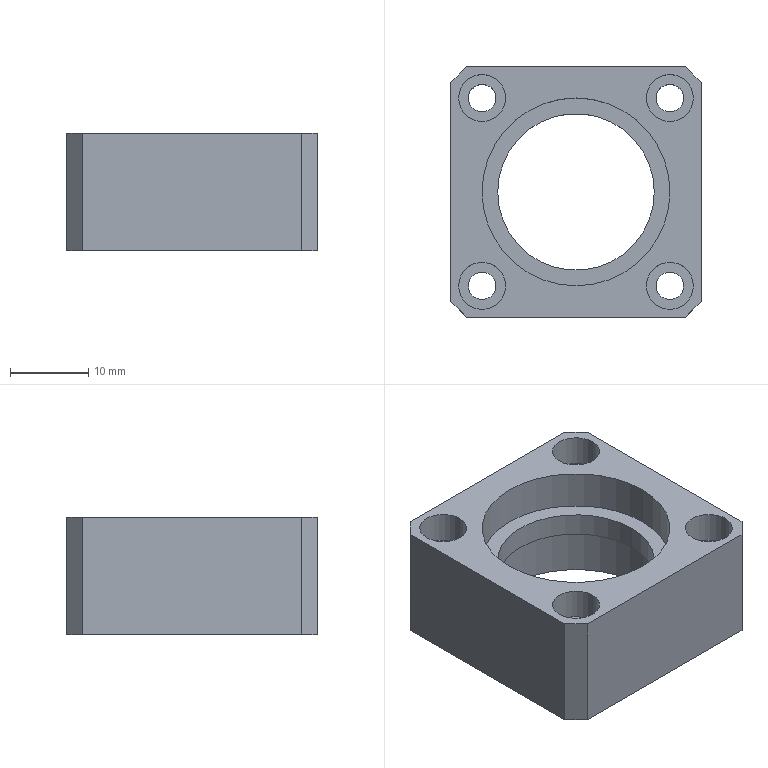Part | SolidWorks | features ICE 3, Chamfer 1, Extrusion 1, HoleWzd 1 | 1 solid | 38 faces | box 32 x 32 x 15 mm | volume 7993 mm3 | cylinder 22 | plane 16 | commonest cylinder face diameters 3.5 x8 6 x8 24 x4 20 x2
STEP:
#1=CARTESIAN_POINT('',(-15.,12.,3.5));
#2=VERTEX_POINT('',#1);
#3=CARTESIAN_POINT('',(-9.,12.,3.5));
#4=VERTEX_POINT('',#3);
#5=CARTESIAN_POINT('',(-12.,12.,3.5));
#6=DIRECTION('',(0.,0.,1.));
#7=DIRECTION('',(1.,0.,0.));
#8=AXIS2_PLACEMENT_3D('',#5,#6,#7);
#9=CIRCLE('',#8,3.);
#10=EDGE_CURVE('',#2,#4,#9,.T.);
#11=ORIENTED_EDGE('',*,*,#10,.F.);
#12=CARTESIAN_POINT('',(-15.,12.,7.5));
#13=VERTEX_POINT('',#12);
#14=CARTESIAN_POINT('',(-15.,12.,7.5));
#15=DIRECTION('',(0.,0.,1.));
#16=VECTOR('',#15,1000.);
#17=LINE('',#14,#16);
#18=EDGE_CURVE('',#2,#13,#17,.T.);
#19=ORIENTED_EDGE('',*,*,#18,.T.);
#20=CARTESIAN_POINT('',(-9.,12.,7.5));
#21=VERTEX_POINT('',#20);
#22=CARTESIAN_POINT('',(-12.,12.,7.5));
#23=DIRECTION('',(0.,0.,1.));
#24=DIRECTION('',(1.,0.,0.));
#25=AXIS2_PLACEMENT_3D('',#22,#23,#24);
#26=CIRCLE('',#25,3.);
#27=EDGE_CURVE('',#13,#21,#26,.T.);
#28=ORIENTED_EDGE('',*,*,#27,.T.);
#29=CARTESIAN_POINT('',(-9.,12.,7.5));
#30=DIRECTION('',(0.,0.,1.));
#31=VECTOR('',#30,1000.);
#32=LINE('',#29,#31);
#33=EDGE_CURVE('',#4,#21,#32,.T.);
#34=ORIENTED_EDGE('',*,*,#33,.F.);
#35=EDGE_LOOP('',(#11,#19,#28,#34));
#36=FACE_OUTER_BOUND('',#35,.T.);
#37=CARTESIAN_POINT('',(-12.,12.,7.5));
#38=DIRECTION('',(0.,0.,1.));
#39=DIRECTION('',(1.,0.,0.));
#40=AXIS2_PLACEMENT_3D('',#37,#38,#39);
#41=CYLINDRICAL_SURFACE('',#40,3.);
#42=ADVANCED_FACE('',(#36),#41,.F.);
#43=CARTESIAN_POINT('',(-13.75,12.,-7.5));
#44=VERTEX_POINT('',#43);
#45=CARTESIAN_POINT('',(-10.25,12.,-7.5));
#46=VERTEX_POINT('',#45);
#47=CARTESIAN_POINT('',(-12.,12.,-7.5));
#48=DIRECTION('',(0.,0.,1.));
#49=DIRECTION('',(1.,0.,0.));
#50=AXIS2_PLACEMENT_3D('',#47,#48,#49);
#51=CIRCLE('',#50,1.75);
#52=EDGE_CURVE('',#44,#46,#51,.T.);
#53=ORIENTED_EDGE('',*,*,#52,.F.);
#54=CARTESIAN_POINT('',(-13.75,12.,3.5));
#55=VERTEX_POINT('',#54);
#56=CARTESIAN_POINT('',(-13.75,12.,7.5));
#57=DIRECTION('',(0.,0.,1.));
#58=VECTOR('',#57,1000.);
#59=LINE('',#56,#58);
#60=EDGE_CURVE('',#44,#55,#59,.T.);
#61=ORIENTED_EDGE('',*,*,#60,.T.);
#62=CARTESIAN_POINT('',(-10.25,12.,3.5));
#63=VERTEX_POINT('',#62);
#64=CARTESIAN_POINT('',(-12.,12.,3.5));
#65=DIRECTION('',(0.,0.,1.));
#66=DIRECTION('',(1.,0.,0.));
#67=AXIS2_PLACEMENT_3D('',#64,#65,#66);
#68=CIRCLE('',#67,1.75);
#69=EDGE_CURVE('',#55,#63,#68,.T.);
#70=ORIENTED_EDGE('',*,*,#69,.T.);
#71=CARTESIAN_POINT('',(-10.25,12.,7.5));
#72=DIRECTION('',(0.,0.,1.));
#73=VECTOR('',#72,1000.);
#74=LINE('',#71,#73);
#75=EDGE_CURVE('',#46,#63,#74,.T.);
#76=ORIENTED_EDGE('',*,*,#75,.F.);
#77=EDGE_LOOP('',(#53,#61,#70,#76));
#78=FACE_OUTER_BOUND('',#77,.T.);
#79=CARTESIAN_POINT('',(-12.,12.,7.5));
#80=DIRECTION('',(0.,0.,1.));
#81=DIRECTION('',(1.,0.,0.));
#82=AXIS2_PLACEMENT_3D('',#79,#80,#81);
#83=CYLINDRICAL_SURFACE('',#82,1.75);
#84=ADVANCED_FACE('',(#78),#83,.F.);
#85=CARTESIAN_POINT('',(9.,12.,3.5));
#86=VERTEX_POINT('',#85);
#87=CARTESIAN_POINT('',(15.,12.,3.5));
#88=VERTEX_POINT('',#87);
#89=CARTESIAN_POINT('',(12.,12.,3.5));
#90=DIRECTION('',(0.,0.,1.));
#91=DIRECTION('',(1.,0.,0.));
#92=AXIS2_PLACEMENT_3D('',#89,#90,#91);
#93=CIRCLE('',#92,3.);
#94=EDGE_CURVE('',#86,#88,#93,.T.);
#95=ORIENTED_EDGE('',*,*,#94,.F.);
#96=CARTESIAN_POINT('',(9.,12.,7.5));
#97=VERTEX_POINT('',#96);
#98=CARTESIAN_POINT('',(9.,12.,7.5));
#99=DIRECTION('',(0.,0.,1.));
#100=VECTOR('',#99,1000.);
#101=LINE('',#98,#100);
#102=EDGE_CURVE('',#86,#97,#101,.T.);
#103=ORIENTED_EDGE('',*,*,#102,.T.);
#104=CARTESIAN_POINT('',(15.,12.,7.5));
#105=VERTEX_POINT('',#104);
#106=CARTESIAN_POINT('',(12.,12.,7.5));
#107=DIRECTION('',(0.,0.,1.));
#108=DIRECTION('',(1.,0.,0.));
#109=AXIS2_PLACEMENT_3D('',#106,#107,#108);
#110=CIRCLE('',#109,3.);
#111=EDGE_CURVE('',#97,#105,#110,.T.);
#112=ORIENTED_EDGE('',*,*,#111,.T.);
#113=CARTESIAN_POINT('',(15.,12.,7.5));
#114=DIRECTION('',(0.,0.,1.));
#115=VECTOR('',#114,1000.);
#116=LINE('',#113,#115);
#117=EDGE_CURVE('',#88,#105,#116,.T.);
#118=ORIENTED_EDGE('',*,*,#117,.F.);
#119=EDGE_LOOP('',(#95,#103,#112,#118));
#120=FACE_OUTER_BOUND('',#119,.T.);
#121=CARTESIAN_POINT('',(12.,12.,7.5));
#122=DIRECTION('',(0.,0.,1.));
#123=DIRECTION('',(1.,0.,0.));
#124=AXIS2_PLACEMENT_3D('',#121,#122,#123);
#125=CYLINDRICAL_SURFACE('',#124,3.);
#126=ADVANCED_FACE('',(#120),#125,.F.);
#127=CARTESIAN_POINT('',(10.25,12.,-7.5));
#128=VERTEX_POINT('',#127);
#129=CARTESIAN_POINT('',(13.75,12.,-7.5));
#130=VERTEX_POINT('',#129);
#131=CARTESIAN_POINT('',(12.,12.,-7.5));
#132=DIRECTION('',(0.,0.,1.));
#133=DIRECTION('',(1.,0.,0.));
#134=AXIS2_PLACEMENT_3D('',#131,#132,#133);
#135=CIRCLE('',#134,1.75);
#136=EDGE_CURVE('',#128,#130,#135,.T.);
#137=ORIENTED_EDGE('',*,*,#136,.F.);
#138=CARTESIAN_POINT('',(10.25,12.,3.5));
#139=VERTEX_POINT('',#138);
#140=CARTESIAN_POINT('',(10.25,12.,7.5));
#141=DIRECTION('',(0.,0.,1.));
#142=VECTOR('',#141,1000.);
#143=LINE('',#140,#142);
#144=EDGE_CURVE('',#128,#139,#143,.T.);
#145=ORIENTED_EDGE('',*,*,#144,.T.);
#146=CARTESIAN_POINT('',(13.75,12.,3.5));
#147=VERTEX_POINT('',#146);
#148=CARTESIAN_POINT('',(12.,12.,3.5));
#149=DIRECTION('',(0.,0.,1.));
#150=DIRECTION('',(1.,0.,0.));
#151=AXIS2_PLACEMENT_3D('',#148,#149,#150);
#152=CIRCLE('',#151,1.75);
#153=EDGE_CURVE('',#139,#147,#152,.T.);
#154=ORIENTED_EDGE('',*,*,#153,.T.);
#155=CARTESIAN_POINT('',(13.75,12.,7.5));
#156=DIRECTION('',(0.,0.,1.));
#157=VECTOR('',#156,1000.);
#158=LINE('',#155,#157);
#159=EDGE_CURVE('',#130,#147,#158,.T.);
#160=ORIENTED_EDGE('',*,*,#159,.F.);
#161=EDGE_LOOP('',(#137,#145,#154,#160));
#162=FACE_OUTER_BOUND('',#161,.T.);
#163=CARTESIAN_POINT('',(12.,12.,7.5));
#164=DIRECTION('',(0.,0.,1.));
#165=DIRECTION('',(1.,0.,0.));
#166=AXIS2_PLACEMENT_3D('',#163,#164,#165);
#167=CYLINDRICAL_SURFACE('',#166,1.75);
#168=ADVANCED_FACE('',(#162),#167,.F.);
#169=CARTESIAN_POINT('',(9.,-12.,3.5));
#170=VERTEX_POINT('',#169);
#171=CARTESIAN_POINT('',(15.,-12.,3.5));
#172=VERTEX_POINT('',#171);
#173=CARTESIAN_POINT('',(12.,-12.,3.5));
#174=DIRECTION('',(0.,0.,1.));
#175=DIRECTION('',(1.,0.,0.));
#176=AXIS2_PLACEMENT_3D('',#173,#174,#175);
#177=CIRCLE('',#176,3.);
#178=EDGE_CURVE('',#170,#172,#177,.T.);
#179=ORIENTED_EDGE('',*,*,#178,.F.);
#180=CARTESIAN_POINT('',(9.,-12.,7.5));
#181=VERTEX_POINT('',#180);
#182=CARTESIAN_POINT('',(9.,-12.,7.5));
#183=DIRECTION('',(0.,0.,1.));
#184=VECTOR('',#183,1000.);
#185=LINE('',#182,#184);
#186=EDGE_CURVE('',#170,#181,#185,.T.);
#187=ORIENTED_EDGE('',*,*,#186,.T.);
#188=CARTESIAN_POINT('',(15.,-12.,7.5));
#189=VERTEX_POINT('',#188);
#190=CARTESIAN_POINT('',(12.,-12.,7.5));
#191=DIRECTION('',(0.,0.,1.));
#192=DIRECTION('',(1.,0.,0.));
#193=AXIS2_PLACEMENT_3D('',#190,#191,#192);
#194=CIRCLE('',#193,3.);
#195=EDGE_CURVE('',#181,#189,#194,.T.);
#196=ORIENTED_EDGE('',*,*,#195,.T.);
#197=CARTESIAN_POINT('',(15.,-12.,7.5));
#198=DIRECTION('',(0.,0.,1.));
#199=VECTOR('',#198,1000.);
#200=LINE('',#197,#199);
#201=EDGE_CURVE('',#172,#189,#200,.T.);
#202=ORIENTED_EDGE('',*,*,#201,.F.);
#203=EDGE_LOOP('',(#179,#187,#196,#202));
#204=FACE_OUTER_BOUND('',#203,.T.);
#205=CARTESIAN_POINT('',(12.,-12.,7.5));
#206=DIRECTION('',(0.,0.,1.));
#207=DIRECTION('',(1.,0.,0.));
#208=AXIS2_PLACEMENT_3D('',#205,#206,#207);
#209=CYLINDRICAL_SURFACE('',#208,3.);
#210=ADVANCED_FACE('',(#204),#209,.F.);
#211=CARTESIAN_POINT('',(10.25,-12.,-7.5));
#212=VERTEX_POINT('',#211);
#213=CARTESIAN_POINT('',(13.75,-12.,-7.5));
#214=VERTEX_POINT('',#213);
#215=CARTESIAN_POINT('',(12.,-12.,-7.5));
#216=DIRECTION('',(0.,0.,1.));
#217=DIRECTION('',(1.,0.,0.));
#218=AXIS2_PLACEMENT_3D('',#215,#216,#217);
#219=CIRCLE('',#218,1.75);
#220=EDGE_CURVE('',#212,#214,#219,.T.);
#221=ORIENTED_EDGE('',*,*,#220,.F.);
#222=CARTESIAN_POINT('',(10.25,-12.,3.5));
#223=VERTEX_POINT('',#222);
#224=CARTESIAN_POINT('',(10.25,-12.,7.5));
#225=DIRECTION('',(0.,0.,1.));
#226=VECTOR('',#225,1000.);
#227=LINE('',#224,#226);
#228=EDGE_CURVE('',#212,#223,#227,.T.);
#229=ORIENTED_EDGE('',*,*,#228,.T.);
#230=CARTESIAN_POINT('',(13.75,-12.,3.5));
#231=VERTEX_POINT('',#230);
#232=CARTESIAN_POINT('',(12.,-12.,3.5));
#233=DIRECTION('',(0.,0.,1.));
#234=DIRECTION('',(1.,0.,0.));
#235=AXIS2_PLACEMENT_3D('',#232,#233,#234);
#236=CIRCLE('',#235,1.75);
#237=EDGE_CURVE('',#223,#231,#236,.T.);
#238=ORIENTED_EDGE('',*,*,#237,.T.);
#239=CARTESIAN_POINT('',(13.75,-12.,7.5));
#240=DIRECTION('',(0.,0.,1.));
#241=VECTOR('',#240,1000.);
#242=LINE('',#239,#241);
#243=EDGE_CURVE('',#214,#231,#242,.T.);
#244=ORIENTED_EDGE('',*,*,#243,.F.);
#245=EDGE_LOOP('',(#221,#229,#238,#244));
#246=FACE_OUTER_BOUND('',#245,.T.);
#247=CARTESIAN_POINT('',(12.,-12.,7.5));
#248=DIRECTION('',(0.,0.,1.));
#249=DIRECTION('',(1.,0.,0.));
#250=AXIS2_PLACEMENT_3D('',#247,#248,#249);
#251=CYLINDRICAL_SURFACE('',#250,1.75);
#252=ADVANCED_FACE('',(#246),#251,.F.);
#253=CARTESIAN_POINT('',(-15.,-12.,3.5));
#254=VERTEX_POINT('',#253);
#255=CARTESIAN_POINT('',(-9.,-12.,3.5));
#256=VERTEX_POINT('',#255);
#257=CARTESIAN_POINT('',(-12.,-12.,3.5));
#258=DIRECTION('',(0.,0.,1.));
#259=DIRECTION('',(1.,0.,0.));
#260=AXIS2_PLACEMENT_3D('',#257,#258,#259);
#261=CIRCLE('',#260,3.);
#262=EDGE_CURVE('',#254,#256,#261,.T.);
#263=ORIENTED_EDGE('',*,*,#262,.F.);
#264=CARTESIAN_POINT('',(-15.,-12.,7.5));
#265=VERTEX_POINT('',#264);
#266=CARTESIAN_POINT('',(-15.,-12.,7.5));
#267=DIRECTION('',(0.,0.,1.));
#268=VECTOR('',#267,1000.);
#269=LINE('',#266,#268);
#270=EDGE_CURVE('',#254,#265,#269,.T.);
#271=ORIENTED_EDGE('',*,*,#270,.T.);
#272=CARTESIAN_POINT('',(-9.,-12.,7.5));
#273=VERTEX_POINT('',#272);
#274=CARTESIAN_POINT('',(-12.,-12.,7.5));
#275=DIRECTION('',(0.,0.,1.));
#276=DIRECTION('',(1.,0.,0.));
#277=AXIS2_PLACEMENT_3D('',#274,#275,#276);
#278=CIRCLE('',#277,3.);
#279=EDGE_CURVE('',#265,#273,#278,.T.);
#280=ORIENTED_EDGE('',*,*,#279,.T.);
#281=CARTESIAN_POINT('',(-9.,-12.,7.5));
#282=DIRECTION('',(0.,0.,1.));
#283=VECTOR('',#282,1000.);
#284=LINE('',#281,#283);
#285=EDGE_CURVE('',#256,#273,#284,.T.);
#286=ORIENTED_EDGE('',*,*,#285,.F.);
#287=EDGE_LOOP('',(#263,#271,#280,#286));
#288=FACE_OUTER_BOUND('',#287,.T.);
#289=CARTESIAN_POINT('',(-12.,-12.,7.5));
#290=DIRECTION('',(0.,0.,1.));
#291=DIRECTION('',(1.,0.,0.));
#292=AXIS2_PLACEMENT_3D('',#289,#290,#291);
#293=CYLINDRICAL_SURFACE('',#292,3.);
#294=ADVANCED_FACE('',(#288),#293,.F.);
#295=CARTESIAN_POINT('',(-13.75,-12.,-7.5));
#296=VERTEX_POINT('',#295);
#297=CARTESIAN_POINT('',(-10.25,-12.,-7.5));
#298=VERTEX_POINT('',#297);
#299=CARTESIAN_POINT('',(-12.,-12.,-7.5));
#300=DIRECTION('',(0.,0.,1.));
#301=DIRECTION('',(1.,0.,0.));
#302=AXIS2_PLACEMENT_3D('',#299,#300,#301);
#303=CIRCLE('',#302,1.75);
#304=EDGE_CURVE('',#296,#298,#303,.T.);
#305=ORIENTED_EDGE('',*,*,#304,.F.);
#306=CARTESIAN_POINT('',(-13.75,-12.,3.5));
#307=VERTEX_POINT('',#306);
#308=CARTESIAN_POINT('',(-13.75,-12.,7.5));
#309=DIRECTION('',(0.,0.,1.));
#310=VECTOR('',#309,1000.);
#311=LINE('',#308,#310);
#312=EDGE_CURVE('',#296,#307,#311,.T.);
#313=ORIENTED_EDGE('',*,*,#312,.T.);
#314=CARTESIAN_POINT('',(-10.25,-12.,3.5));
#315=VERTEX_POINT('',#314);
#316=CARTESIAN_POINT('',(-12.,-12.,3.5));
#317=DIRECTION('',(0.,0.,1.));
#318=DIRECTION('',(1.,0.,0.));
#319=AXIS2_PLACEMENT_3D('',#316,#317,#318);
#320=CIRCLE('',#319,1.75);
#321=EDGE_CURVE('',#307,#315,#320,.T.);
#322=ORIENTED_EDGE('',*,*,#321,.T.);
#323=CARTESIAN_POINT('',(-10.25,-12.,7.5));
#324=DIRECTION('',(0.,0.,1.));
#325=VECTOR('',#324,1000.);
#326=LINE('',#323,#325);
#327=EDGE_CURVE('',#298,#315,#326,.T.);
#328=ORIENTED_EDGE('',*,*,#327,.F.);
#329=EDGE_LOOP('',(#305,#313,#322,#328));
#330=FACE_OUTER_BOUND('',#329,.T.);
#331=CARTESIAN_POINT('',(-12.,-12.,7.5));
#332=DIRECTION('',(0.,0.,1.));
#333=DIRECTION('',(1.,0.,0.));
#334=AXIS2_PLACEMENT_3D('',#331,#332,#333);
#335=CYLINDRICAL_SURFACE('',#334,1.75);
#336=ADVANCED_FACE('',(#330),#335,.F.);
#337=CARTESIAN_POINT('',(12.,0.,-0.5));
#338=VERTEX_POINT('',#337);
#339=CARTESIAN_POINT('',(-12.,0.,-0.5));
#340=VERTEX_POINT('',#339);
#341=CARTESIAN_POINT('',(0.,0.,-0.5));
#342=DIRECTION('',(0.,0.,-1.));
#343=DIRECTION('',(-1.,0.,0.));
#344=AXIS2_PLACEMENT_3D('',#341,#342,#343);
#345=CIRCLE('',#344,12.);
#346=EDGE_CURVE('',#338,#340,#345,.T.);
#347=ORIENTED_EDGE('',*,*,#346,.F.);
#348=CARTESIAN_POINT('',(12.,0.,-7.5));
#349=VERTEX_POINT('',#348);
#350=CARTESIAN_POINT('',(12.,0.,-0.5));
#351=DIRECTION('',(0.,0.,-1.));
#352=VECTOR('',#351,1000.);
#353=LINE('',#350,#352);
#354=EDGE_CURVE('',#338,#349,#353,.T.);
#355=ORIENTED_EDGE('',*,*,#354,.T.);
#356=CARTESIAN_POINT('',(-12.,0.,-7.5));
#357=VERTEX_POINT('',#356);
#358=CARTESIAN_POINT('',(0.,0.,-7.5));
#359=DIRECTION('',(0.,0.,-1.));
#360=DIRECTION('',(-1.,0.,0.));
#361=AXIS2_PLACEMENT_3D('',#358,#359,#360);
#362=CIRCLE('',#361,12.);
#363=EDGE_CURVE('',#349,#357,#362,.T.);
#364=ORIENTED_EDGE('',*,*,#363,.T.);
#365=CARTESIAN_POINT('',(-12.,0.,-0.5));
#366=DIRECTION('',(0.,0.,-1.));
#367=VECTOR('',#366,1000.);
#368=LINE('',#365,#367);
#369=EDGE_CURVE('',#340,#357,#368,.T.);
#370=ORIENTED_EDGE('',*,*,#369,.F.);
#371=EDGE_LOOP('',(#347,#355,#364,#370));
#372=FACE_OUTER_BOUND('',#371,.T.);
#373=CARTESIAN_POINT('',(0.,0.,-0.5));
#374=DIRECTION('',(0.,0.,-1.));
#375=DIRECTION('',(-1.,0.,0.));
#376=AXIS2_PLACEMENT_3D('',#373,#374,#375);
#377=CYLINDRICAL_SURFACE('',#376,12.);
#378=ADVANCED_FACE('',(#372),#377,.F.);
#379=CARTESIAN_POINT('',(-12.,0.,2.5));
#380=VERTEX_POINT('',#379);
#381=CARTESIAN_POINT('',(12.,0.,2.5));
#382=VERTEX_POINT('',#381);
#383=CARTESIAN_POINT('',(0.,0.,2.5));
#384=DIRECTION('',(0.,0.,1.));
#385=DIRECTION('',(1.,0.,0.));
#386=AXIS2_PLACEMENT_3D('',#383,#384,#385);
#387=CIRCLE('',#386,12.);
#388=EDGE_CURVE('',#380,#382,#387,.T.);
#389=ORIENTED_EDGE('',*,*,#388,.F.);
#390=CARTESIAN_POINT('',(-12.,0.,7.5));
#391=VERTEX_POINT('',#390);
#392=CARTESIAN_POINT('',(-12.,0.,2.5));
#393=DIRECTION('',(0.,0.,1.));
#394=VECTOR('',#393,1000.);
#395=LINE('',#392,#394);
#396=EDGE_CURVE('',#380,#391,#395,.T.);
#397=ORIENTED_EDGE('',*,*,#396,.T.);
#398=CARTESIAN_POINT('',(12.,0.,7.5));
#399=VERTEX_POINT('',#398);
#400=CARTESIAN_POINT('',(0.,0.,7.5));
#401=DIRECTION('',(0.,0.,1.));
#402=DIRECTION('',(1.,0.,0.));
#403=AXIS2_PLACEMENT_3D('',#400,#401,#402);
#404=CIRCLE('',#403,12.);
#405=EDGE_CURVE('',#391,#399,#404,.T.);
#406=ORIENTED_EDGE('',*,*,#405,.T.);
#407=CARTESIAN_POINT('',(12.,0.,2.5));
#408=DIRECTION('',(0.,0.,1.));
#409=VECTOR('',#408,1000.);
#410=LINE('',#407,#409);
#411=EDGE_CURVE('',#382,#399,#410,.T.);
#412=ORIENTED_EDGE('',*,*,#411,.F.);
#413=EDGE_LOOP('',(#389,#397,#406,#412));
#414=FACE_OUTER_BOUND('',#413,.T.);
#415=CARTESIAN_POINT('',(0.,0.,2.5));
#416=DIRECTION('',(0.,0.,1.));
#417=DIRECTION('',(1.,0.,0.));
#418=AXIS2_PLACEMENT_3D('',#415,#416,#417);
#419=CYLINDRICAL_SURFACE('',#418,12.);
#420=ADVANCED_FACE('',(#414),#419,.F.);
#421=CARTESIAN_POINT('',(-10.,0.,-0.5));
#422=VERTEX_POINT('',#421);
#423=CARTESIAN_POINT('',(10.,0.,-0.5));
#424=VERTEX_POINT('',#423);
#425=CARTESIAN_POINT('',(0.,0.,-0.5));
#426=DIRECTION('',(0.,0.,1.));
#427=DIRECTION('',(-1.,0.,0.));
#428=AXIS2_PLACEMENT_3D('',#425,#426,#427);
#429=CIRCLE('',#428,10.);
#430=EDGE_CURVE('',#422,#424,#429,.T.);
#431=ORIENTED_EDGE('',*,*,#430,.F.);
#432=CARTESIAN_POINT('',(-10.,0.,2.5));
#433=VERTEX_POINT('',#432);
#434=CARTESIAN_POINT('',(-10.,0.,-7.5));
#435=DIRECTION('',(0.,0.,1.));
#436=VECTOR('',#435,1000.);
#437=LINE('',#434,#436);
#438=EDGE_CURVE('',#422,#433,#437,.T.);
#439=ORIENTED_EDGE('',*,*,#438,.T.);
#440=CARTESIAN_POINT('',(10.,0.,2.5));
#441=VERTEX_POINT('',#440);
#442=CARTESIAN_POINT('',(0.,0.,2.5));
#443=DIRECTION('',(0.,0.,-1.));
#444=DIRECTION('',(1.,0.,0.));
#445=AXIS2_PLACEMENT_3D('',#442,#443,#444);
#446=CIRCLE('',#445,10.);
#447=EDGE_CURVE('',#441,#433,#446,.T.);
#448=ORIENTED_EDGE('',*,*,#447,.F.);
#449=CARTESIAN_POINT('',(10.,0.,-7.5));
#450=DIRECTION('',(0.,0.,1.));
#451=VECTOR('',#450,1000.);
#452=LINE('',#449,#451);
#453=EDGE_CURVE('',#424,#441,#452,.T.);
#454=ORIENTED_EDGE('',*,*,#453,.F.);
#455=EDGE_LOOP('',(#431,#439,#448,#454));
#456=FACE_OUTER_BOUND('',#455,.T.);
#457=CARTESIAN_POINT('',(0.,0.,-7.5));
#458=DIRECTION('',(0.,0.,1.));
#459=DIRECTION('',(1.,0.,0.));
#460=AXIS2_PLACEMENT_3D('',#457,#458,#459);
#461=CYLINDRICAL_SURFACE('',#460,10.);
#462=ADVANCED_FACE('',(#456),#461,.F.);
#463=ORIENTED_EDGE('',*,*,#438,.F.);
#464=CARTESIAN_POINT('',(0.,0.,-0.5));
#465=DIRECTION('',(0.,0.,1.));
#466=DIRECTION('',(-1.,0.,0.));
#467=AXIS2_PLACEMENT_3D('',#464,#465,#466);
#468=CIRCLE('',#467,10.);
#469=EDGE_CURVE('',#424,#422,#468,.T.);
#470=ORIENTED_EDGE('',*,*,#469,.F.);
#471=ORIENTED_EDGE('',*,*,#453,.T.);
#472=CARTESIAN_POINT('',(0.,0.,2.5));
#473=DIRECTION('',(0.,0.,-1.));
#474=DIRECTION('',(1.,0.,0.));
#475=AXIS2_PLACEMENT_3D('',#472,#473,#474);
#476=CIRCLE('',#475,10.);
#477=EDGE_CURVE('',#433,#441,#476,.T.);
#478=ORIENTED_EDGE('',*,*,#477,.F.);
#479=EDGE_LOOP('',(#463,#470,#471,#478));
#480=FACE_OUTER_BOUND('',#479,.T.);
#481=CARTESIAN_POINT('',(0.,0.,-7.5));
#482=DIRECTION('',(0.,0.,1.));
#483=DIRECTION('',(1.,0.,0.));
#484=AXIS2_PLACEMENT_3D('',#481,#482,#483);
#485=CYLINDRICAL_SURFACE('',#484,10.);
#486=ADVANCED_FACE('',(#480),#485,.F.);
#487=CARTESIAN_POINT('',(16.,-14.,7.5));
#488=VERTEX_POINT('',#487);
#489=CARTESIAN_POINT('',(16.,14.,7.5));
#490=VERTEX_POINT('',#489);
#491=CARTESIAN_POINT('',(16.,16.,7.5));
#492=DIRECTION('',(0.,1.,0.));
#493=VECTOR('',#492,1000.);
#494=LINE('',#491,#493);
#495=EDGE_CURVE('',#488,#490,#494,.T.);
#496=ORIENTED_EDGE('',*,*,#495,.F.);
#497=CARTESIAN_POINT('',(16.,-14.,-7.5));
#498=VERTEX_POINT('',#497);
#499=CARTESIAN_POINT('',(16.,-14.,7.5));
#500=DIRECTION('',(0.,0.,-1.));
#501=VECTOR('',#500,1000.);
#502=LINE('',#499,#501);
#503=EDGE_CURVE('',#488,#498,#502,.T.);
#504=ORIENTED_EDGE('',*,*,#503,.T.);
#505=CARTESIAN_POINT('',(16.,14.,-7.5));
#506=VERTEX_POINT('',#505);
#507=CARTESIAN_POINT('',(16.,16.,-7.5));
#508=DIRECTION('',(0.,1.,0.));
#509=VECTOR('',#508,1000.);
#510=LINE('',#507,#509);
#511=EDGE_CURVE('',#498,#506,#510,.T.);
#512=ORIENTED_EDGE('',*,*,#511,.T.);
#513=CARTESIAN_POINT('',(16.,14.,7.5));
#514=DIRECTION('',(0.,0.,1.));
#515=VECTOR('',#514,1000.);
#516=LINE('',#513,#515);
#517=EDGE_CURVE('',#506,#490,#516,.T.);
#518=ORIENTED_EDGE('',*,*,#517,.T.);
#519=EDGE_LOOP('',(#496,#504,#512,#518));
#520=FACE_OUTER_BOUND('',#519,.T.);
#521=CARTESIAN_POINT('',(16.,16.,7.5));
#522=DIRECTION('',(-1.,0.,0.));
#523=DIRECTION('',(0.,-1.,0.));
#524=AXIS2_PLACEMENT_3D('',#521,#522,#523);
#525=PLANE('',#524);
#526=ADVANCED_FACE('',(#520),#525,.F.);
#527=CARTESIAN_POINT('',(14.,16.,7.5));
#528=VERTEX_POINT('',#527);
#529=CARTESIAN_POINT('',(-14.,16.,7.5));
#530=VERTEX_POINT('',#529);
#531=CARTESIAN_POINT('',(-16.,16.,7.5));
#532=DIRECTION('',(-1.,0.,0.));
#533=VECTOR('',#532,1000.);
#534=LINE('',#531,#533);
#535=EDGE_CURVE('',#528,#530,#534,.T.);
#536=ORIENTED_EDGE('',*,*,#535,.F.);
#537=CARTESIAN_POINT('',(14.,16.,-7.5));
#538=VERTEX_POINT('',#537);
#539=CARTESIAN_POINT('',(14.,16.,7.5));
#540=DIRECTION('',(0.,0.,-1.));
#541=VECTOR('',#540,1000.);
#542=LINE('',#539,#541);
#543=EDGE_CURVE('',#528,#538,#542,.T.);
#544=ORIENTED_EDGE('',*,*,#543,.T.);
#545=CARTESIAN_POINT('',(-14.,16.,-7.5));
#546=VERTEX_POINT('',#545);
#547=CARTESIAN_POINT('',(-16.,16.,-7.5));
#548=DIRECTION('',(-1.,0.,0.));
#549=VECTOR('',#548,1000.);
#550=LINE('',#547,#549);
#551=EDGE_CURVE('',#538,#546,#550,.T.);
#552=ORIENTED_EDGE('',*,*,#551,.T.);
#553=CARTESIAN_POINT('',(-14.,16.,7.5));
#554=DIRECTION('',(0.,0.,1.));
#555=VECTOR('',#554,1000.);
#556=LINE('',#553,#555);
#557=EDGE_CURVE('',#546,#530,#556,.T.);
#558=ORIENTED_EDGE('',*,*,#557,.T.);
#559=EDGE_LOOP('',(#536,#544,#552,#558));
#560=FACE_OUTER_BOUND('',#559,.T.);
#561=CARTESIAN_POINT('',(-16.,16.,7.5));
#562=DIRECTION('',(0.,-1.,0.));
#563=DIRECTION('',(0.,0.,-1.));
#564=AXIS2_PLACEMENT_3D('',#561,#562,#563);
#565=PLANE('',#564);
#566=ADVANCED_FACE('',(#560),#565,.F.);
#567=CARTESIAN_POINT('',(-16.,14.,-7.5));
#568=VERTEX_POINT('',#567);
#569=CARTESIAN_POINT('',(-16.,-14.,-7.5));
#570=VERTEX_POINT('',#569);
#571=CARTESIAN_POINT('',(-16.,16.,-7.5));
#572=DIRECTION('',(0.,-1.,0.));
#573=VECTOR('',#572,1000.);
#574=LINE('',#571,#573);
#575=EDGE_CURVE('',#568,#570,#574,.T.);
#576=ORIENTED_EDGE('',*,*,#575,.T.);
#577=CARTESIAN_POINT('',(-16.,-14.,7.5));
#578=VERTEX_POINT('',#577);
#579=CARTESIAN_POINT('',(-16.,-14.,7.5));
#580=DIRECTION('',(0.,0.,1.));
#581=VECTOR('',#580,1000.);
#582=LINE('',#579,#581);
#583=EDGE_CURVE('',#570,#578,#582,.T.);
#584=ORIENTED_EDGE('',*,*,#583,.T.);
#585=CARTESIAN_POINT('',(-16.,14.,7.5));
#586=VERTEX_POINT('',#585);
#587=CARTESIAN_POINT('',(-16.,16.,7.5));
#588=DIRECTION('',(0.,-1.,0.));
#589=VECTOR('',#588,1000.);
#590=LINE('',#587,#589);
#591=EDGE_CURVE('',#586,#578,#590,.T.);
#592=ORIENTED_EDGE('',*,*,#591,.F.);
#593=CARTESIAN_POINT('',(-16.,14.,7.5));
#594=DIRECTION('',(0.,0.,-1.));
#595=VECTOR('',#594,1000.);
#596=LINE('',#593,#595);
#597=EDGE_CURVE('',#586,#568,#596,.T.);
#598=ORIENTED_EDGE('',*,*,#597,.T.);
#599=EDGE_LOOP('',(#576,#584,#592,#598));
#600=FACE_OUTER_BOUND('',#599,.T.);
#601=CARTESIAN_POINT('',(-16.,16.,7.5));
#602=DIRECTION('',(1.,0.,0.));
#603=DIRECTION('',(0.,1.,0.));
#604=AXIS2_PLACEMENT_3D('',#601,#602,#603);
#605=PLANE('',#604);
#606=ADVANCED_FACE('',(#600),#605,.F.);
#607=CARTESIAN_POINT('',(-14.,-16.,7.5));
#608=VERTEX_POINT('',#607);
#609=CARTESIAN_POINT('',(14.,-16.,7.5));
#610=VERTEX_POINT('',#609);
#611=CARTESIAN_POINT('',(-16.,-16.,7.5));
#612=DIRECTION('',(1.,0.,0.));
#613=VECTOR('',#612,1000.);
#614=LINE('',#611,#613);
#615=EDGE_CURVE('',#608,#610,#614,.T.);
#616=ORIENTED_EDGE('',*,*,#615,.F.);
#617=CARTESIAN_POINT('',(-14.,-16.,-7.5));
#618=VERTEX_POINT('',#617);
#619=CARTESIAN_POINT('',(-14.,-16.,7.5));
#620=DIRECTION('',(0.,0.,-1.));
#621=VECTOR('',#620,1000.);
#622=LINE('',#619,#621);
#623=EDGE_CURVE('',#608,#618,#622,.T.);
#624=ORIENTED_EDGE('',*,*,#623,.T.);
#625=CARTESIAN_POINT('',(14.,-16.,-7.5));
#626=VERTEX_POINT('',#625);
#627=CARTESIAN_POINT('',(-16.,-16.,-7.5));
#628=DIRECTION('',(1.,0.,0.));
#629=VECTOR('',#628,1000.);
#630=LINE('',#627,#629);
#631=EDGE_CURVE('',#618,#626,#630,.T.);
#632=ORIENTED_EDGE('',*,*,#631,.T.);
#633=CARTESIAN_POINT('',(14.,-16.,7.5));
#634=DIRECTION('',(0.,0.,1.));
#635=VECTOR('',#634,1000.);
#636=LINE('',#633,#635);
#637=EDGE_CURVE('',#626,#610,#636,.T.);
#638=ORIENTED_EDGE('',*,*,#637,.T.);
#639=EDGE_LOOP('',(#616,#624,#632,#638));
#640=FACE_OUTER_BOUND('',#639,.T.);
#641=CARTESIAN_POINT('',(-16.,-16.,7.5));
#642=DIRECTION('',(0.,1.,0.));
#643=DIRECTION('',(-1.,0.,0.));
#644=AXIS2_PLACEMENT_3D('',#641,#642,#643);
#645=PLANE('',#644);
#646=ADVANCED_FACE('',(#640),#645,.F.);
#647=CARTESIAN_POINT('',(-12.,12.,7.5));
#648=DIRECTION('',(0.,0.,1.));
#649=DIRECTION('',(1.,0.,0.));
#650=AXIS2_PLACEMENT_3D('',#647,#648,#649);
#651=CIRCLE('',#650,3.);
#652=EDGE_CURVE('',#21,#13,#651,.T.);
#653=ORIENTED_EDGE('',*,*,#652,.F.);
#654=ORIENTED_EDGE('',*,*,#27,.F.);
#655=EDGE_LOOP('',(#653,#654));
#656=FACE_BOUND('',#655,.T.);
#657=CARTESIAN_POINT('',(12.,12.,7.5));
#658=DIRECTION('',(0.,0.,1.));
#659=DIRECTION('',(1.,0.,0.));
#660=AXIS2_PLACEMENT_3D('',#657,#658,#659);
#661=CIRCLE('',#660,3.);
#662=EDGE_CURVE('',#105,#97,#661,.T.);
#663=ORIENTED_EDGE('',*,*,#662,.F.);
#664=ORIENTED_EDGE('',*,*,#111,.F.);
#665=EDGE_LOOP('',(#663,#664));
#666=FACE_BOUND('',#665,.T.);
#667=CARTESIAN_POINT('',(12.,-12.,7.5));
#668=DIRECTION('',(0.,0.,1.));
#669=DIRECTION('',(1.,0.,0.));
#670=AXIS2_PLACEMENT_3D('',#667,#668,#669);
#671=CIRCLE('',#670,3.);
#672=EDGE_CURVE('',#189,#181,#671,.T.);
#673=ORIENTED_EDGE('',*,*,#672,.F.);
#674=ORIENTED_EDGE('',*,*,#195,.F.);
#675=EDGE_LOOP('',(#673,#674));
#676=FACE_BOUND('',#675,.T.);
#677=CARTESIAN_POINT('',(-12.,-12.,7.5));
#678=DIRECTION('',(0.,0.,1.));
#679=DIRECTION('',(1.,0.,0.));
#680=AXIS2_PLACEMENT_3D('',#677,#678,#679);
#681=CIRCLE('',#680,3.);
#682=EDGE_CURVE('',#273,#265,#681,.T.);
#683=ORIENTED_EDGE('',*,*,#682,.F.);
#684=ORIENTED_EDGE('',*,*,#279,.F.);
#685=EDGE_LOOP('',(#683,#684));
#686=FACE_BOUND('',#685,.T.);
#687=CARTESIAN_POINT('',(0.,0.,7.5));
#688=DIRECTION('',(0.,0.,1.));
#689=DIRECTION('',(1.,0.,0.));
#690=AXIS2_PLACEMENT_3D('',#687,#688,#689);
#691=CIRCLE('',#690,12.);
#692=EDGE_CURVE('',#399,#391,#691,.T.);
#693=ORIENTED_EDGE('',*,*,#692,.F.);
#694=ORIENTED_EDGE('',*,*,#405,.F.);
#695=EDGE_LOOP('',(#693,#694));
#696=FACE_BOUND('',#695,.T.);
#697=ORIENTED_EDGE('',*,*,#591,.T.);
#698=CARTESIAN_POINT('',(-15.,-15.,7.5));
#699=DIRECTION('',(0.7071,-0.7071,0.));
#700=VECTOR('',#699,1000.);
#701=LINE('',#698,#700);
#702=EDGE_CURVE('',#578,#608,#701,.T.);
#703=ORIENTED_EDGE('',*,*,#702,.T.);
#704=ORIENTED_EDGE('',*,*,#615,.T.);
#705=CARTESIAN_POINT('',(15.,-15.,7.5));
#706=DIRECTION('',(0.7071,0.7071,0.));
#707=VECTOR('',#706,1000.);
#708=LINE('',#705,#707);
#709=EDGE_CURVE('',#610,#488,#708,.T.);
#710=ORIENTED_EDGE('',*,*,#709,.T.);
#711=ORIENTED_EDGE('',*,*,#495,.T.);
#712=CARTESIAN_POINT('',(15.,15.,7.5));
#713=DIRECTION('',(-0.7071,0.7071,0.));
#714=VECTOR('',#713,1000.);
#715=LINE('',#712,#714);
#716=EDGE_CURVE('',#490,#528,#715,.T.);
#717=ORIENTED_EDGE('',*,*,#716,.T.);
#718=ORIENTED_EDGE('',*,*,#535,.T.);
#719=CARTESIAN_POINT('',(-15.,15.,7.5));
#720=DIRECTION('',(-0.7071,-0.7071,0.));
#721=VECTOR('',#720,1000.);
#722=LINE('',#719,#721);
#723=EDGE_CURVE('',#530,#586,#722,.T.);
#724=ORIENTED_EDGE('',*,*,#723,.T.);
#725=EDGE_LOOP('',(#697,#703,#704,#710,#711,#717,#718,#724));
#726=FACE_OUTER_BOUND('',#725,.T.);
#727=CARTESIAN_POINT('',(0.,0.,7.5));
#728=DIRECTION('',(0.,0.,1.));
#729=DIRECTION('',(1.,0.,0.));
#730=AXIS2_PLACEMENT_3D('',#727,#728,#729);
#731=PLANE('',#730);
#732=ADVANCED_FACE('',(#656,#666,#676,#686,#696,#726),#731,.T.);
#733=CARTESIAN_POINT('',(-12.,12.,-7.5));
#734=DIRECTION('',(0.,0.,1.));
#735=DIRECTION('',(1.,0.,0.));
#736=AXIS2_PLACEMENT_3D('',#733,#734,#735);
#737=CIRCLE('',#736,1.75);
#738=EDGE_CURVE('',#46,#44,#737,.T.);
#739=ORIENTED_EDGE('',*,*,#738,.T.);
#740=ORIENTED_EDGE('',*,*,#52,.T.);
#741=EDGE_LOOP('',(#739,#740));
#742=FACE_BOUND('',#741,.T.);
#743=CARTESIAN_POINT('',(12.,12.,-7.5));
#744=DIRECTION('',(0.,0.,1.));
#745=DIRECTION('',(1.,0.,0.));
#746=AXIS2_PLACEMENT_3D('',#743,#744,#745);
#747=CIRCLE('',#746,1.75);
#748=EDGE_CURVE('',#130,#128,#747,.T.);
#749=ORIENTED_EDGE('',*,*,#748,.T.);
#750=ORIENTED_EDGE('',*,*,#136,.T.);
#751=EDGE_LOOP('',(#749,#750));
#752=FACE_BOUND('',#751,.T.);
#753=CARTESIAN_POINT('',(12.,-12.,-7.5));
#754=DIRECTION('',(0.,0.,1.));
#755=DIRECTION('',(1.,0.,0.));
#756=AXIS2_PLACEMENT_3D('',#753,#754,#755);
#757=CIRCLE('',#756,1.75);
#758=EDGE_CURVE('',#214,#212,#757,.T.);
#759=ORIENTED_EDGE('',*,*,#758,.T.);
#760=ORIENTED_EDGE('',*,*,#220,.T.);
#761=EDGE_LOOP('',(#759,#760));
#762=FACE_BOUND('',#761,.T.);
#763=CARTESIAN_POINT('',(-12.,-12.,-7.5));
#764=DIRECTION('',(0.,0.,1.));
#765=DIRECTION('',(1.,0.,0.));
#766=AXIS2_PLACEMENT_3D('',#763,#764,#765);
#767=CIRCLE('',#766,1.75);
#768=EDGE_CURVE('',#298,#296,#767,.T.);
#769=ORIENTED_EDGE('',*,*,#768,.T.);
#770=ORIENTED_EDGE('',*,*,#304,.T.);
#771=EDGE_LOOP('',(#769,#770));
#772=FACE_BOUND('',#771,.T.);
#773=CARTESIAN_POINT('',(0.,0.,-7.5));
#774=DIRECTION('',(0.,0.,-1.));
#775=DIRECTION('',(-1.,0.,0.));
#776=AXIS2_PLACEMENT_3D('',#773,#774,#775);
#777=CIRCLE('',#776,12.);
#778=EDGE_CURVE('',#357,#349,#777,.T.);
#779=ORIENTED_EDGE('',*,*,#778,.F.);
#780=ORIENTED_EDGE('',*,*,#363,.F.);
#781=EDGE_LOOP('',(#779,#780));
#782=FACE_BOUND('',#781,.T.);
#783=ORIENTED_EDGE('',*,*,#631,.F.);
#784=CARTESIAN_POINT('',(-14.,-16.,-7.5));
#785=DIRECTION('',(-0.7071,0.7071,0.));
#786=VECTOR('',#785,1000.);
#787=LINE('',#784,#786);
#788=EDGE_CURVE('',#618,#570,#787,.T.);
#789=ORIENTED_EDGE('',*,*,#788,.T.);
#790=ORIENTED_EDGE('',*,*,#575,.F.);
#791=CARTESIAN_POINT('',(-16.,14.,-7.5));
#792=DIRECTION('',(0.7071,0.7071,0.));
#793=VECTOR('',#792,1000.);
#794=LINE('',#791,#793);
#795=EDGE_CURVE('',#568,#546,#794,.T.);
#796=ORIENTED_EDGE('',*,*,#795,.T.);
#797=ORIENTED_EDGE('',*,*,#551,.F.);
#798=CARTESIAN_POINT('',(14.,16.,-7.5));
#799=DIRECTION('',(0.7071,-0.7071,0.));
#800=VECTOR('',#799,1000.);
#801=LINE('',#798,#800);
#802=EDGE_CURVE('',#538,#506,#801,.T.);
#803=ORIENTED_EDGE('',*,*,#802,.T.);
#804=ORIENTED_EDGE('',*,*,#511,.F.);
#805=CARTESIAN_POINT('',(16.,-14.,-7.5));
#806=DIRECTION('',(-0.7071,-0.7071,0.));
#807=VECTOR('',#806,1000.);
#808=LINE('',#805,#807);
#809=EDGE_CURVE('',#498,#626,#808,.T.);
#810=ORIENTED_EDGE('',*,*,#809,.T.);
#811=EDGE_LOOP('',(#783,#789,#790,#796,#797,#803,#804,#810));
#812=FACE_OUTER_BOUND('',#811,.T.);
#813=CARTESIAN_POINT('',(0.,0.,-7.5));
#814=DIRECTION('',(0.,0.,1.));
#815=DIRECTION('',(1.,0.,0.));
#816=AXIS2_PLACEMENT_3D('',#813,#814,#815);
#817=PLANE('',#816);
#818=ADVANCED_FACE('',(#742,#752,#762,#772,#782,#812),#817,.F.);
#819=CARTESIAN_POINT('',(0.,0.,2.5));
#820=DIRECTION('',(0.,0.,1.));
#821=DIRECTION('',(1.,0.,0.));
#822=AXIS2_PLACEMENT_3D('',#819,#820,#821);
#823=CIRCLE('',#822,12.);
#824=EDGE_CURVE('',#382,#380,#823,.T.);
#825=ORIENTED_EDGE('',*,*,#824,.T.);
#826=ORIENTED_EDGE('',*,*,#388,.T.);
#827=EDGE_LOOP('',(#825,#826));
#828=FACE_OUTER_BOUND('',#827,.T.);
#829=ORIENTED_EDGE('',*,*,#447,.T.);
#830=ORIENTED_EDGE('',*,*,#477,.T.);
#831=EDGE_LOOP('',(#829,#830));
#832=FACE_BOUND('',#831,.T.);
#833=CARTESIAN_POINT('',(0.,0.,2.5));
#834=DIRECTION('',(0.,0.,1.));
#835=DIRECTION('',(1.,0.,0.));
#836=AXIS2_PLACEMENT_3D('',#833,#834,#835);
#837=PLANE('',#836);
#838=ADVANCED_FACE('',(#828,#832),#837,.T.);
#839=ORIENTED_EDGE('',*,*,#396,.F.);
#840=ORIENTED_EDGE('',*,*,#824,.F.);
#841=ORIENTED_EDGE('',*,*,#411,.T.);
#842=ORIENTED_EDGE('',*,*,#692,.T.);
#843=EDGE_LOOP('',(#839,#840,#841,#842));
#844=FACE_OUTER_BOUND('',#843,.T.);
#845=CARTESIAN_POINT('',(0.,0.,2.5));
#846=DIRECTION('',(0.,0.,1.));
#847=DIRECTION('',(1.,0.,0.));
#848=AXIS2_PLACEMENT_3D('',#845,#846,#847);
#849=CYLINDRICAL_SURFACE('',#848,12.);
#850=ADVANCED_FACE('',(#844),#849,.F.);
#851=CARTESIAN_POINT('',(0.,0.,-0.5));
#852=DIRECTION('',(0.,0.,-1.));
#853=DIRECTION('',(-1.,0.,0.));
#854=AXIS2_PLACEMENT_3D('',#851,#852,#853);
#855=CIRCLE('',#854,12.);
#856=EDGE_CURVE('',#340,#338,#855,.T.);
#857=ORIENTED_EDGE('',*,*,#856,.T.);
#858=ORIENTED_EDGE('',*,*,#346,.T.);
#859=EDGE_LOOP('',(#857,#858));
#860=FACE_OUTER_BOUND('',#859,.T.);
#861=ORIENTED_EDGE('',*,*,#469,.T.);
#862=ORIENTED_EDGE('',*,*,#430,.T.);
#863=EDGE_LOOP('',(#861,#862));
#864=FACE_BOUND('',#863,.T.);
#865=CARTESIAN_POINT('',(0.,0.,-0.5));
#866=DIRECTION('',(0.,0.,-1.));
#867=DIRECTION('',(-1.,0.,0.));
#868=AXIS2_PLACEMENT_3D('',#865,#866,#867);
#869=PLANE('',#868);
#870=ADVANCED_FACE('',(#860,#864),#869,.T.);
#871=ORIENTED_EDGE('',*,*,#354,.F.);
#872=ORIENTED_EDGE('',*,*,#856,.F.);
#873=ORIENTED_EDGE('',*,*,#369,.T.);
#874=ORIENTED_EDGE('',*,*,#778,.T.);
#875=EDGE_LOOP('',(#871,#872,#873,#874));
#876=FACE_OUTER_BOUND('',#875,.T.);
#877=CARTESIAN_POINT('',(0.,0.,-0.5));
#878=DIRECTION('',(0.,0.,-1.));
#879=DIRECTION('',(-1.,0.,0.));
#880=AXIS2_PLACEMENT_3D('',#877,#878,#879);
#881=CYLINDRICAL_SURFACE('',#880,12.);
#882=ADVANCED_FACE('',(#876),#881,.F.);
#883=ORIENTED_EDGE('',*,*,#702,.F.);
#884=ORIENTED_EDGE('',*,*,#583,.F.);
#885=ORIENTED_EDGE('',*,*,#788,.F.);
#886=ORIENTED_EDGE('',*,*,#623,.F.);
#887=EDGE_LOOP('',(#883,#884,#885,#886));
#888=FACE_OUTER_BOUND('',#887,.T.);
#889=CARTESIAN_POINT('',(-14.,-16.,7.5));
#890=DIRECTION('',(0.7071,0.7071,0.));
#891=DIRECTION('',(0.,0.,-1.));
#892=AXIS2_PLACEMENT_3D('',#889,#890,#891);
#893=PLANE('',#892);
#894=ADVANCED_FACE('',(#888),#893,.F.);
#895=ORIENTED_EDGE('',*,*,#709,.F.);
#896=ORIENTED_EDGE('',*,*,#637,.F.);
#897=ORIENTED_EDGE('',*,*,#809,.F.);
#898=ORIENTED_EDGE('',*,*,#503,.F.);
#899=EDGE_LOOP('',(#895,#896,#897,#898));
#900=FACE_OUTER_BOUND('',#899,.T.);
#901=CARTESIAN_POINT('',(16.,-14.,7.5));
#902=DIRECTION('',(-0.7071,0.7071,0.));
#903=DIRECTION('',(0.,0.,-1.));
#904=AXIS2_PLACEMENT_3D('',#901,#902,#903);
#905=PLANE('',#904);
#906=ADVANCED_FACE('',(#900),#905,.F.);
#907=ORIENTED_EDGE('',*,*,#716,.F.);
#908=ORIENTED_EDGE('',*,*,#517,.F.);
#909=ORIENTED_EDGE('',*,*,#802,.F.);
#910=ORIENTED_EDGE('',*,*,#543,.F.);
#911=EDGE_LOOP('',(#907,#908,#909,#910));
#912=FACE_OUTER_BOUND('',#911,.T.);
#913=CARTESIAN_POINT('',(14.,16.,7.5));
#914=DIRECTION('',(-0.7071,-0.7071,0.));
#915=DIRECTION('',(0.,0.,-1.));
#916=AXIS2_PLACEMENT_3D('',#913,#914,#915);
#917=PLANE('',#916);
#918=ADVANCED_FACE('',(#912),#917,.F.);
#919=ORIENTED_EDGE('',*,*,#723,.F.);
#920=ORIENTED_EDGE('',*,*,#557,.F.);
#921=ORIENTED_EDGE('',*,*,#795,.F.);
#922=ORIENTED_EDGE('',*,*,#597,.F.);
#923=EDGE_LOOP('',(#919,#920,#921,#922));
#924=FACE_OUTER_BOUND('',#923,.T.);
#925=CARTESIAN_POINT('',(-16.,14.,7.5));
#926=DIRECTION('',(0.7071,-0.7071,0.));
#927=DIRECTION('',(0.,0.,-1.));
#928=AXIS2_PLACEMENT_3D('',#925,#926,#927);
#929=PLANE('',#928);
#930=ADVANCED_FACE('',(#924),#929,.F.);
#931=ORIENTED_EDGE('',*,*,#312,.F.);
#932=ORIENTED_EDGE('',*,*,#768,.F.);
#933=ORIENTED_EDGE('',*,*,#327,.T.);
#934=CARTESIAN_POINT('',(-12.,-12.,3.5));
#935=DIRECTION('',(0.,0.,1.));
#936=DIRECTION('',(1.,0.,0.));
#937=AXIS2_PLACEMENT_3D('',#934,#935,#936);
#938=CIRCLE('',#937,1.75);
#939=EDGE_CURVE('',#315,#307,#938,.T.);
#940=ORIENTED_EDGE('',*,*,#939,.T.);
#941=EDGE_LOOP('',(#931,#932,#933,#940));
#942=FACE_OUTER_BOUND('',#941,.T.);
#943=CARTESIAN_POINT('',(-12.,-12.,7.5));
#944=DIRECTION('',(0.,0.,1.));
#945=DIRECTION('',(1.,0.,0.));
#946=AXIS2_PLACEMENT_3D('',#943,#944,#945);
#947=CYLINDRICAL_SURFACE('',#946,1.75);
#948=ADVANCED_FACE('',(#942),#947,.F.);
#949=ORIENTED_EDGE('',*,*,#939,.F.);
#950=ORIENTED_EDGE('',*,*,#321,.F.);
#951=EDGE_LOOP('',(#949,#950));
#952=FACE_BOUND('',#951,.T.);
#953=CARTESIAN_POINT('',(-12.,-12.,3.5));
#954=DIRECTION('',(0.,0.,1.));
#955=DIRECTION('',(1.,0.,0.));
#956=AXIS2_PLACEMENT_3D('',#953,#954,#955);
#957=CIRCLE('',#956,3.);
#958=EDGE_CURVE('',#256,#254,#957,.T.);
#959=ORIENTED_EDGE('',*,*,#958,.T.);
#960=ORIENTED_EDGE('',*,*,#262,.T.);
#961=EDGE_LOOP('',(#959,#960));
#962=FACE_OUTER_BOUND('',#961,.T.);
#963=CARTESIAN_POINT('',(-10.25,-12.,3.5));
#964=DIRECTION('',(0.,0.,-1.));
#965=DIRECTION('',(-1.,0.,0.));
#966=AXIS2_PLACEMENT_3D('',#963,#964,#965);
#967=PLANE('',#966);
#968=ADVANCED_FACE('',(#952,#962),#967,.F.);
#969=ORIENTED_EDGE('',*,*,#270,.F.);
#970=ORIENTED_EDGE('',*,*,#958,.F.);
#971=ORIENTED_EDGE('',*,*,#285,.T.);
#972=ORIENTED_EDGE('',*,*,#682,.T.);
#973=EDGE_LOOP('',(#969,#970,#971,#972));
#974=FACE_OUTER_BOUND('',#973,.T.);
#975=CARTESIAN_POINT('',(-12.,-12.,7.5));
#976=DIRECTION('',(0.,0.,1.));
#977=DIRECTION('',(1.,0.,0.));
#978=AXIS2_PLACEMENT_3D('',#975,#976,#977);
#979=CYLINDRICAL_SURFACE('',#978,3.);
#980=ADVANCED_FACE('',(#974),#979,.F.);
#981=ORIENTED_EDGE('',*,*,#228,.F.);
#982=ORIENTED_EDGE('',*,*,#758,.F.);
#983=ORIENTED_EDGE('',*,*,#243,.T.);
#984=CARTESIAN_POINT('',(12.,-12.,3.5));
#985=DIRECTION('',(0.,0.,1.));
#986=DIRECTION('',(1.,0.,0.));
#987=AXIS2_PLACEMENT_3D('',#984,#985,#986);
#988=CIRCLE('',#987,1.75);
#989=EDGE_CURVE('',#231,#223,#988,.T.);
#990=ORIENTED_EDGE('',*,*,#989,.T.);
#991=EDGE_LOOP('',(#981,#982,#983,#990));
#992=FACE_OUTER_BOUND('',#991,.T.);
#993=CARTESIAN_POINT('',(12.,-12.,7.5));
#994=DIRECTION('',(0.,0.,1.));
#995=DIRECTION('',(1.,0.,0.));
#996=AXIS2_PLACEMENT_3D('',#993,#994,#995);
#997=CYLINDRICAL_SURFACE('',#996,1.75);
#998=ADVANCED_FACE('',(#992),#997,.F.);
#999=ORIENTED_EDGE('',*,*,#989,.F.);
#1000=ORIENTED_EDGE('',*,*,#237,.F.);
#1001=EDGE_LOOP('',(#999,#1000));
#1002=FACE_BOUND('',#1001,.T.);
#1003=CARTESIAN_POINT('',(12.,-12.,3.5));
#1004=DIRECTION('',(0.,0.,1.));
#1005=DIRECTION('',(1.,0.,0.));
#1006=AXIS2_PLACEMENT_3D('',#1003,#1004,#1005);
#1007=CIRCLE('',#1006,3.);
#1008=EDGE_CURVE('',#172,#170,#1007,.T.);
#1009=ORIENTED_EDGE('',*,*,#1008,.T.);
#1010=ORIENTED_EDGE('',*,*,#178,.T.);
#1011=EDGE_LOOP('',(#1009,#1010));
#1012=FACE_OUTER_BOUND('',#1011,.T.);
#1013=CARTESIAN_POINT('',(13.75,-12.,3.5));
#1014=DIRECTION('',(0.,0.,-1.));
#1015=DIRECTION('',(-1.,0.,0.));
#1016=AXIS2_PLACEMENT_3D('',#1013,#1014,#1015);
#1017=PLANE('',#1016);
#1018=ADVANCED_FACE('',(#1002,#1012),#1017,.F.);
#1019=ORIENTED_EDGE('',*,*,#186,.F.);
#1020=ORIENTED_EDGE('',*,*,#1008,.F.);
#1021=ORIENTED_EDGE('',*,*,#201,.T.);
#1022=ORIENTED_EDGE('',*,*,#672,.T.);
#1023=EDGE_LOOP('',(#1019,#1020,#1021,#1022));
#1024=FACE_OUTER_BOUND('',#1023,.T.);
#1025=CARTESIAN_POINT('',(12.,-12.,7.5));
#1026=DIRECTION('',(0.,0.,1.));
#1027=DIRECTION('',(1.,0.,0.));
#1028=AXIS2_PLACEMENT_3D('',#1025,#1026,#1027);
#1029=CYLINDRICAL_SURFACE('',#1028,3.);
#1030=ADVANCED_FACE('',(#1024),#1029,.F.);
#1031=ORIENTED_EDGE('',*,*,#144,.F.);
#1032=ORIENTED_EDGE('',*,*,#748,.F.);
#1033=ORIENTED_EDGE('',*,*,#159,.T.);
#1034=CARTESIAN_POINT('',(12.,12.,3.5));
#1035=DIRECTION('',(0.,0.,1.));
#1036=DIRECTION('',(1.,0.,0.));
#1037=AXIS2_PLACEMENT_3D('',#1034,#1035,#1036);
#1038=CIRCLE('',#1037,1.75);
#1039=EDGE_CURVE('',#147,#139,#1038,.T.);
#1040=ORIENTED_EDGE('',*,*,#1039,.T.);
#1041=EDGE_LOOP('',(#1031,#1032,#1033,#1040));
#1042=FACE_OUTER_BOUND('',#1041,.T.);
#1043=CARTESIAN_POINT('',(12.,12.,7.5));
#1044=DIRECTION('',(0.,0.,1.));
#1045=DIRECTION('',(1.,0.,0.));
#1046=AXIS2_PLACEMENT_3D('',#1043,#1044,#1045);
#1047=CYLINDRICAL_SURFACE('',#1046,1.75);
#1048=ADVANCED_FACE('',(#1042),#1047,.F.);
#1049=ORIENTED_EDGE('',*,*,#1039,.F.);
#1050=ORIENTED_EDGE('',*,*,#153,.F.);
#1051=EDGE_LOOP('',(#1049,#1050));
#1052=FACE_BOUND('',#1051,.T.);
#1053=CARTESIAN_POINT('',(12.,12.,3.5));
#1054=DIRECTION('',(0.,0.,1.));
#1055=DIRECTION('',(1.,0.,0.));
#1056=AXIS2_PLACEMENT_3D('',#1053,#1054,#1055);
#1057=CIRCLE('',#1056,3.);
#1058=EDGE_CURVE('',#88,#86,#1057,.T.);
#1059=ORIENTED_EDGE('',*,*,#1058,.T.);
#1060=ORIENTED_EDGE('',*,*,#94,.T.);
#1061=EDGE_LOOP('',(#1059,#1060));
#1062=FACE_OUTER_BOUND('',#1061,.T.);
#1063=CARTESIAN_POINT('',(13.75,12.,3.5));
#1064=DIRECTION('',(0.,0.,-1.));
#1065=DIRECTION('',(-1.,0.,0.));
#1066=AXIS2_PLACEMENT_3D('',#1063,#1064,#1065);
#1067=PLANE('',#1066);
#1068=ADVANCED_FACE('',(#1052,#1062),#1067,.F.);
#1069=ORIENTED_EDGE('',*,*,#102,.F.);
#1070=ORIENTED_EDGE('',*,*,#1058,.F.);
#1071=ORIENTED_EDGE('',*,*,#117,.T.);
#1072=ORIENTED_EDGE('',*,*,#662,.T.);
#1073=EDGE_LOOP('',(#1069,#1070,#1071,#1072));
#1074=FACE_OUTER_BOUND('',#1073,.T.);
#1075=CARTESIAN_POINT('',(12.,12.,7.5));
#1076=DIRECTION('',(0.,0.,1.));
#1077=DIRECTION('',(1.,0.,0.));
#1078=AXIS2_PLACEMENT_3D('',#1075,#1076,#1077);
#1079=CYLINDRICAL_SURFACE('',#1078,3.);
#1080=ADVANCED_FACE('',(#1074),#1079,.F.);
#1081=ORIENTED_EDGE('',*,*,#60,.F.);
#1082=ORIENTED_EDGE('',*,*,#738,.F.);
#1083=ORIENTED_EDGE('',*,*,#75,.T.);
#1084=CARTESIAN_POINT('',(-12.,12.,3.5));
#1085=DIRECTION('',(0.,0.,1.));
#1086=DIRECTION('',(1.,0.,0.));
#1087=AXIS2_PLACEMENT_3D('',#1084,#1085,#1086);
#1088=CIRCLE('',#1087,1.75);
#1089=EDGE_CURVE('',#63,#55,#1088,.T.);
#1090=ORIENTED_EDGE('',*,*,#1089,.T.);
#1091=EDGE_LOOP('',(#1081,#1082,#1083,#1090));
#1092=FACE_OUTER_BOUND('',#1091,.T.);
#1093=CARTESIAN_POINT('',(-12.,12.,7.5));
#1094=DIRECTION('',(0.,0.,1.));
#1095=DIRECTION('',(1.,0.,0.));
#1096=AXIS2_PLACEMENT_3D('',#1093,#1094,#1095);
#1097=CYLINDRICAL_SURFACE('',#1096,1.75);
#1098=ADVANCED_FACE('',(#1092),#1097,.F.);
#1099=ORIENTED_EDGE('',*,*,#1089,.F.);
#1100=ORIENTED_EDGE('',*,*,#69,.F.);
#1101=EDGE_LOOP('',(#1099,#1100));
#1102=FACE_BOUND('',#1101,.T.);
#1103=CARTESIAN_POINT('',(-12.,12.,3.5));
#1104=DIRECTION('',(0.,0.,1.));
#1105=DIRECTION('',(1.,0.,0.));
#1106=AXIS2_PLACEMENT_3D('',#1103,#1104,#1105);
#1107=CIRCLE('',#1106,3.);
#1108=EDGE_CURVE('',#4,#2,#1107,.T.);
#1109=ORIENTED_EDGE('',*,*,#1108,.T.);
#1110=ORIENTED_EDGE('',*,*,#10,.T.);
#1111=EDGE_LOOP('',(#1109,#1110));
#1112=FACE_OUTER_BOUND('',#1111,.T.);
#1113=CARTESIAN_POINT('',(-10.25,12.,3.5));
#1114=DIRECTION('',(0.,0.,-1.));
#1115=DIRECTION('',(-1.,0.,0.));
#1116=AXIS2_PLACEMENT_3D('',#1113,#1114,#1115);
#1117=PLANE('',#1116);
#1118=ADVANCED_FACE('',(#1102,#1112),#1117,.F.);
#1119=ORIENTED_EDGE('',*,*,#18,.F.);
#1120=ORIENTED_EDGE('',*,*,#1108,.F.);
#1121=ORIENTED_EDGE('',*,*,#33,.T.);
#1122=ORIENTED_EDGE('',*,*,#652,.T.);
#1123=EDGE_LOOP('',(#1119,#1120,#1121,#1122));
#1124=FACE_OUTER_BOUND('',#1123,.T.);
#1125=CARTESIAN_POINT('',(-12.,12.,7.5));
#1126=DIRECTION('',(0.,0.,1.));
#1127=DIRECTION('',(1.,0.,0.));
#1128=AXIS2_PLACEMENT_3D('',#1125,#1126,#1127);
#1129=CYLINDRICAL_SURFACE('',#1128,3.);
#1130=ADVANCED_FACE('',(#1124),#1129,.F.);
#1131=CLOSED_SHELL('',(#42,#84,#126,#168,#210,#252,#294,#336,#378,#420,#462,#486,#526,#566,#606,#646,#732,#818,#838,#850,#870,#882,#894,#906,#918,#930,#948,#968,#980,#998,#1018,#1030,#1048,#1068,#1080,#1098,#1118,#1130));
#1132=MANIFOLD_SOLID_BREP('',#1131);
#1133=CARTESIAN_POINT('',(0.,0.,0.));
#1134=DIRECTION('',(0.,0.,1.));
#1135=DIRECTION('',(1.,0.,0.));
#1136=AXIS2_PLACEMENT_3D('',#1133,#1134,#1135);
#1137=(LENGTH_UNIT()NAMED_UNIT(*)SI_UNIT(.MILLI.,.METRE.));
#1138=UNCERTAINTY_MEASURE_WITH_UNIT(LENGTH_MEASURE(0.00001),#1137,'','');
#1139=(NAMED_UNIT(*)PLANE_ANGLE_UNIT()SI_UNIT($,.RADIAN.));
#1140=(NAMED_UNIT(*)SI_UNIT($,.STERADIAN.)SOLID_ANGLE_UNIT());
#1141=(GEOMETRIC_REPRESENTATION_CONTEXT(3)GLOBAL_UNCERTAINTY_ASSIGNED_CONTEXT((#1138))GLOBAL_UNIT_ASSIGNED_CONTEXT((#1137,#1139,#1140))REPRESENTATION_CONTEXT('',''));
#1142=ADVANCED_BREP_SHAPE_REPRESENTATION('',(#1132,#1136),#1141);